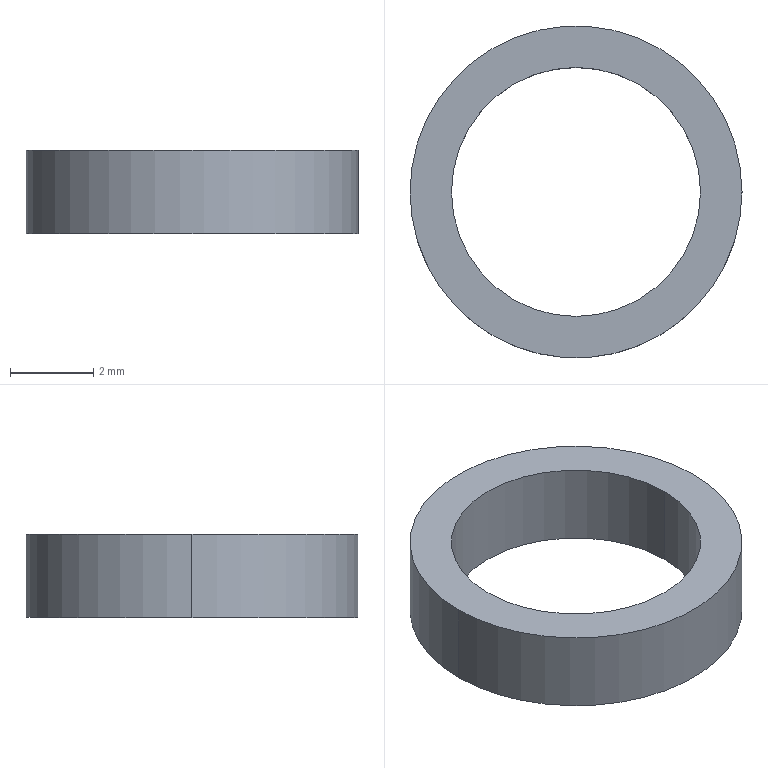Part | SolidWorks | features Extrusion 1 | 1 solid | 6 faces | box 8 x 8 x 2 mm | volume 43.982 mm3 | cylinder 4 | plane 2 | commonest cylinder face diameters 6 x2 8 x2
STEP:
#1=CARTESIAN_POINT('',(-3.,0.,2.));
#2=VERTEX_POINT('',#1);
#3=CARTESIAN_POINT('',(3.,0.,2.));
#4=VERTEX_POINT('',#3);
#5=CARTESIAN_POINT('',(0.,0.,2.));
#6=DIRECTION('',(0.,0.,1.));
#7=DIRECTION('',(1.,0.,0.));
#8=AXIS2_PLACEMENT_3D('',#5,#6,#7);
#9=CIRCLE('',#8,3.);
#10=EDGE_CURVE('',#2,#4,#9,.T.);
#11=ORIENTED_EDGE('',*,*,#10,.T.);
#12=CARTESIAN_POINT('',(3.,0.,0.));
#13=VERTEX_POINT('',#12);
#14=CARTESIAN_POINT('',(3.,0.,2.));
#15=DIRECTION('',(0.,0.,-1.));
#16=VECTOR('',#15,1000.);
#17=LINE('',#14,#16);
#18=EDGE_CURVE('',#4,#13,#17,.T.);
#19=ORIENTED_EDGE('',*,*,#18,.T.);
#20=CARTESIAN_POINT('',(-3.,0.,0.));
#21=VERTEX_POINT('',#20);
#22=CARTESIAN_POINT('',(0.,0.,0.));
#23=DIRECTION('',(0.,0.,1.));
#24=DIRECTION('',(1.,0.,0.));
#25=AXIS2_PLACEMENT_3D('',#22,#23,#24);
#26=CIRCLE('',#25,3.);
#27=EDGE_CURVE('',#21,#13,#26,.T.);
#28=ORIENTED_EDGE('',*,*,#27,.F.);
#29=CARTESIAN_POINT('',(-3.,0.,2.));
#30=DIRECTION('',(0.,0.,-1.));
#31=VECTOR('',#30,1000.);
#32=LINE('',#29,#31);
#33=EDGE_CURVE('',#2,#21,#32,.T.);
#34=ORIENTED_EDGE('',*,*,#33,.F.);
#35=EDGE_LOOP('',(#11,#19,#28,#34));
#36=FACE_OUTER_BOUND('',#35,.T.);
#37=CARTESIAN_POINT('',(0.,0.,2.));
#38=DIRECTION('',(0.,0.,-1.));
#39=DIRECTION('',(-1.,0.,0.));
#40=AXIS2_PLACEMENT_3D('',#37,#38,#39);
#41=CYLINDRICAL_SURFACE('',#40,3.);
#42=ADVANCED_FACE('',(#36),#41,.F.);
#43=CARTESIAN_POINT('',(4.,0.,2.));
#44=VERTEX_POINT('',#43);
#45=CARTESIAN_POINT('',(-4.,0.,2.));
#46=VERTEX_POINT('',#45);
#47=CARTESIAN_POINT('',(0.,0.,2.));
#48=DIRECTION('',(0.,0.,1.));
#49=DIRECTION('',(1.,0.,0.));
#50=AXIS2_PLACEMENT_3D('',#47,#48,#49);
#51=CIRCLE('',#50,4.);
#52=EDGE_CURVE('',#44,#46,#51,.T.);
#53=ORIENTED_EDGE('',*,*,#52,.F.);
#54=CARTESIAN_POINT('',(4.,0.,0.));
#55=VERTEX_POINT('',#54);
#56=CARTESIAN_POINT('',(4.,0.,2.));
#57=DIRECTION('',(0.,0.,-1.));
#58=VECTOR('',#57,1000.);
#59=LINE('',#56,#58);
#60=EDGE_CURVE('',#44,#55,#59,.T.);
#61=ORIENTED_EDGE('',*,*,#60,.T.);
#62=CARTESIAN_POINT('',(-4.,0.,0.));
#63=VERTEX_POINT('',#62);
#64=CARTESIAN_POINT('',(0.,0.,0.));
#65=DIRECTION('',(0.,0.,1.));
#66=DIRECTION('',(1.,0.,0.));
#67=AXIS2_PLACEMENT_3D('',#64,#65,#66);
#68=CIRCLE('',#67,4.);
#69=EDGE_CURVE('',#55,#63,#68,.T.);
#70=ORIENTED_EDGE('',*,*,#69,.T.);
#71=CARTESIAN_POINT('',(-4.,0.,2.));
#72=DIRECTION('',(0.,0.,-1.));
#73=VECTOR('',#72,1000.);
#74=LINE('',#71,#73);
#75=EDGE_CURVE('',#46,#63,#74,.T.);
#76=ORIENTED_EDGE('',*,*,#75,.F.);
#77=EDGE_LOOP('',(#53,#61,#70,#76));
#78=FACE_OUTER_BOUND('',#77,.T.);
#79=CARTESIAN_POINT('',(0.,0.,2.));
#80=DIRECTION('',(0.,0.,-1.));
#81=DIRECTION('',(-1.,0.,0.));
#82=AXIS2_PLACEMENT_3D('',#79,#80,#81);
#83=CYLINDRICAL_SURFACE('',#82,4.);
#84=ADVANCED_FACE('',(#78),#83,.T.);
#85=CARTESIAN_POINT('',(0.,0.,2.));
#86=DIRECTION('',(0.,0.,1.));
#87=DIRECTION('',(1.,0.,0.));
#88=AXIS2_PLACEMENT_3D('',#85,#86,#87);
#89=CIRCLE('',#88,4.);
#90=EDGE_CURVE('',#46,#44,#89,.T.);
#91=ORIENTED_EDGE('',*,*,#90,.T.);
#92=ORIENTED_EDGE('',*,*,#52,.T.);
#93=EDGE_LOOP('',(#91,#92));
#94=FACE_OUTER_BOUND('',#93,.T.);
#95=ORIENTED_EDGE('',*,*,#10,.F.);
#96=CARTESIAN_POINT('',(0.,0.,2.));
#97=DIRECTION('',(0.,0.,1.));
#98=DIRECTION('',(1.,0.,0.));
#99=AXIS2_PLACEMENT_3D('',#96,#97,#98);
#100=CIRCLE('',#99,3.);
#101=EDGE_CURVE('',#4,#2,#100,.T.);
#102=ORIENTED_EDGE('',*,*,#101,.F.);
#103=EDGE_LOOP('',(#95,#102));
#104=FACE_BOUND('',#103,.T.);
#105=CARTESIAN_POINT('',(0.,0.,2.));
#106=DIRECTION('',(0.,0.,1.));
#107=DIRECTION('',(1.,0.,0.));
#108=AXIS2_PLACEMENT_3D('',#105,#106,#107);
#109=PLANE('',#108);
#110=ADVANCED_FACE('',(#94,#104),#109,.T.);
#111=CARTESIAN_POINT('',(0.,0.,0.));
#112=DIRECTION('',(0.,0.,1.));
#113=DIRECTION('',(1.,0.,0.));
#114=AXIS2_PLACEMENT_3D('',#111,#112,#113);
#115=CIRCLE('',#114,4.);
#116=EDGE_CURVE('',#63,#55,#115,.T.);
#117=ORIENTED_EDGE('',*,*,#116,.F.);
#118=ORIENTED_EDGE('',*,*,#69,.F.);
#119=EDGE_LOOP('',(#117,#118));
#120=FACE_OUTER_BOUND('',#119,.T.);
#121=ORIENTED_EDGE('',*,*,#27,.T.);
#122=CARTESIAN_POINT('',(0.,0.,0.));
#123=DIRECTION('',(0.,0.,1.));
#124=DIRECTION('',(1.,0.,0.));
#125=AXIS2_PLACEMENT_3D('',#122,#123,#124);
#126=CIRCLE('',#125,3.);
#127=EDGE_CURVE('',#13,#21,#126,.T.);
#128=ORIENTED_EDGE('',*,*,#127,.T.);
#129=EDGE_LOOP('',(#121,#128));
#130=FACE_BOUND('',#129,.T.);
#131=CARTESIAN_POINT('',(0.,0.,0.));
#132=DIRECTION('',(0.,0.,1.));
#133=DIRECTION('',(1.,0.,0.));
#134=AXIS2_PLACEMENT_3D('',#131,#132,#133);
#135=PLANE('',#134);
#136=ADVANCED_FACE('',(#120,#130),#135,.F.);
#137=ORIENTED_EDGE('',*,*,#60,.F.);
#138=ORIENTED_EDGE('',*,*,#90,.F.);
#139=ORIENTED_EDGE('',*,*,#75,.T.);
#140=ORIENTED_EDGE('',*,*,#116,.T.);
#141=EDGE_LOOP('',(#137,#138,#139,#140));
#142=FACE_OUTER_BOUND('',#141,.T.);
#143=CARTESIAN_POINT('',(0.,0.,2.));
#144=DIRECTION('',(0.,0.,-1.));
#145=DIRECTION('',(-1.,0.,0.));
#146=AXIS2_PLACEMENT_3D('',#143,#144,#145);
#147=CYLINDRICAL_SURFACE('',#146,4.);
#148=ADVANCED_FACE('',(#142),#147,.T.);
#149=ORIENTED_EDGE('',*,*,#18,.F.);
#150=ORIENTED_EDGE('',*,*,#101,.T.);
#151=ORIENTED_EDGE('',*,*,#33,.T.);
#152=ORIENTED_EDGE('',*,*,#127,.F.);
#153=EDGE_LOOP('',(#149,#150,#151,#152));
#154=FACE_OUTER_BOUND('',#153,.T.);
#155=CARTESIAN_POINT('',(0.,0.,2.));
#156=DIRECTION('',(0.,0.,-1.));
#157=DIRECTION('',(-1.,0.,0.));
#158=AXIS2_PLACEMENT_3D('',#155,#156,#157);
#159=CYLINDRICAL_SURFACE('',#158,3.);
#160=ADVANCED_FACE('',(#154),#159,.F.);
#161=CLOSED_SHELL('',(#42,#84,#110,#136,#148,#160));
#162=MANIFOLD_SOLID_BREP('',#161);
#163=CARTESIAN_POINT('',(0.,0.,0.));
#164=DIRECTION('',(0.,0.,1.));
#165=DIRECTION('',(1.,0.,0.));
#166=AXIS2_PLACEMENT_3D('',#163,#164,#165);
#167=(LENGTH_UNIT()NAMED_UNIT(*)SI_UNIT(.MILLI.,.METRE.));
#168=UNCERTAINTY_MEASURE_WITH_UNIT(LENGTH_MEASURE(0.00001),#167,'','');
#169=(NAMED_UNIT(*)PLANE_ANGLE_UNIT()SI_UNIT($,.RADIAN.));
#170=(NAMED_UNIT(*)SI_UNIT($,.STERADIAN.)SOLID_ANGLE_UNIT());
#171=(GEOMETRIC_REPRESENTATION_CONTEXT(3)GLOBAL_UNCERTAINTY_ASSIGNED_CONTEXT((#168))GLOBAL_UNIT_ASSIGNED_CONTEXT((#167,#169,#170))REPRESENTATION_CONTEXT('',''));
#172=ADVANCED_BREP_SHAPE_REPRESENTATION('',(#162,#166),#171);